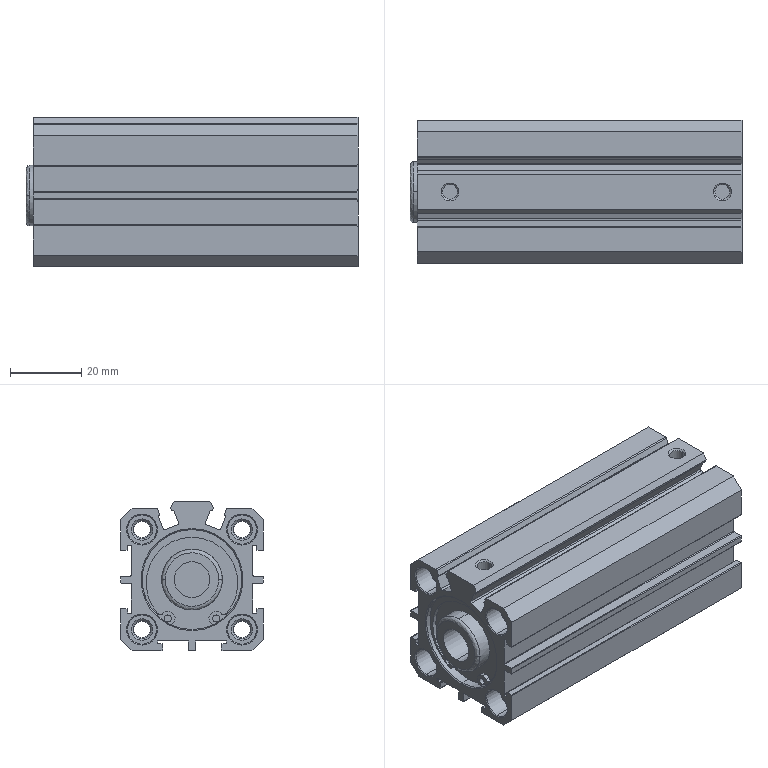Part | STEP file | SDA25x60S-01-cc | 1 solid | 266 faces | box 93 x 40 x 42 mm | volume 80745 mm3 | cylinder 118 | plane 90 | cone 56 | spline 2 | commonest cylinder face diameters 0.4 x46 4.917 x16 8.2 x16 4.6 x8 0.8 x6 2 x6